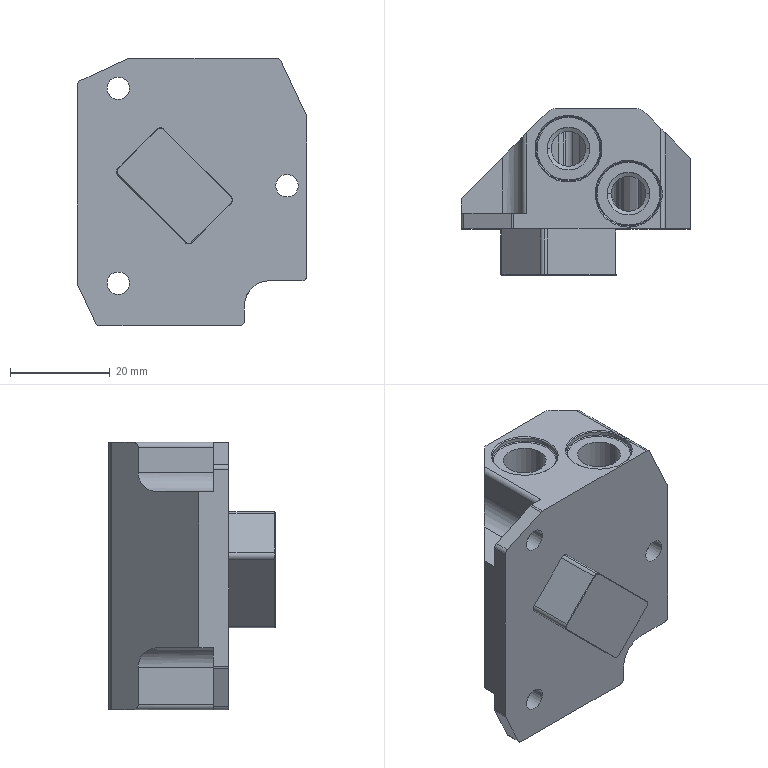NC program | NX | posted with a generic post | part box 46 x 33.25 x 53.5 mm
Lines 4235 to 5331 of 9227:
(CURVE_DRIVE , TOOL : D6R0.5)
N8456 T04 M6
N8458 G53
N8460 G17 G0 G90 X-20.051 Y25.81 B0. C0. S5500 M3
N8462 G43 Z30. H4
N8464 Z-6.42
N8466 G94 G1 Z-7.12 F3000.
N8468 X-20.038 Z-7.382
N8470 X-20.002 Z-7.641
N8472 X-19.944 Z-7.896
N8474 X-19.864 Z-8.145
N8476 X-19.762 Z-8.387
N8478 X-19.64 Z-8.618
N8480 X-19.498 Z-8.838
N8482 X-19.338 Z-9.045
N8484 X-19.16 Z-9.237
N8486 X-18.966 Z-9.412
N8488 X-18.757 Z-9.571
N8490 X-18.536 Z-9.71
N8492 X-18.303 Z-9.829
N8494 X-18.06 Z-9.928
N8496 X-17.81 Z-10.005
N8498 X-17.555 Z-10.061
N8500 X-17.295 Z-10.093
N8502 X-17.033 Z-10.103
N8504 X-3.366
N8506 X-3.309 Y25.792 Z-10.085
N8508 X-3.25 Y25.768 Z-10.061
N8510 X-17.149
N8512 X-17.193 Y25.749 Z-10.042
N8514 X-17.216 Y25.737 Z-10.03
N8516 X-17.234 Y25.726 Z-10.019
N8518 X-3.168 Y25.727 Z-10.02
N8520 X-3.102 Y25.685 Z-9.977
N8522 X-17.302 Y25.684 Z-9.978
N8524 X-17.345 Y25.655 Z-9.948
N8526 X-17.361 Y25.642 Z-9.935
N8528 X-3.043 Y25.643
N8530 X-2.99 Y25.601 Z-9.894
N8532 X-17.412 Y25.6 Z-9.893
N8534 X-17.458 Y25.558 Z-9.851
N8536 X-2.945 Y25.559 Z-9.852
N8538 X-2.918 Y25.532 Z-9.825
N8540 X-2.905 Y25.516 Z-9.81
N8542 X-17.495 Z-9.809
N8544 X-17.531 Y25.474 Z-9.767
N8546 X-2.869
N8548 X-2.855 Y25.456 Z-9.749
N8550 X-2.837 Y25.432 Z-9.725
N8552 X-17.559
N8554 X-17.587 Y25.39 Z-9.683
N8556 X-15.672 Z-9.682
N8558 X-2.809 Z-9.683
N8560 X-2.783 Y25.348 Z-9.641
N8562 X-2.814
N8564 X-17.566 Y25.347
N8566 X-17.615
N8568 X-17.619 Y25.341 Z-9.634
N8570 X-17.638 Y25.305 Z-9.599
N8572 X-17.509 Z-9.598
N8574 X-2.814 Y25.306
N8576 X-2.761 Z-9.599
N8578 X-2.744 Y25.273 Z-9.567
N8580 X-2.74 Y25.263 Z-9.557
N8582 X-2.814 Z-9.556
N8584 X-17.509
N8586 X-17.66
N8588 X-17.676 Y25.221 Z-9.514
N8590 X-17.509
N8592 X-2.814
N8594 X-2.723 Z-9.515
N8596 X-2.715 Y25.202 Z-9.496
N8598 X-2.706 Y25.179 Z-9.474
N8600 X-2.814 Z-9.472
N8602 X-17.509
N8604 X-17.691
N8606 X-17.704 Y25.137 Z-9.43
N8608 X-17.521
N8610 X-2.801
N8612 X-2.695 Z-9.432
N8614 X-2.684 Y25.095 Z-9.389
N8616 X-2.814 Z-9.388
N8618 X-17.558
N8620 X-17.717
N8622 X-17.729 Y25.055 Z-9.348
N8624 X-17.73 Y25.053 Z-9.346
N8626 X-16.499
N8628 X-2.814
N8630 X-2.674 Z-9.347
N8632 X-2.668 Y25.011 Z-9.305
N8634 X-2.814 Z-9.304
N8636 X-17.734
N8638 X-17.739 Y24.968 Z-9.262
N8640 X-2.814 Y24.969
N8642 X-2.662 Z-9.263
N8644 X-2.657 Y24.935 Z-9.229
N8646 Y24.927 Z-9.221
N8648 X-2.814 Z-9.219
N8650 X-17.743 Y24.926
N8652 X-17.745 Y24.884 Z-9.177
N8654 X-2.81
N8656 X-2.655 Z-9.178
N8658 X-2.653 Y24.842 Z-9.136
N8660 X-2.814 Z-9.135
N8662 X-17.747
N8664 X-17.749 Y24.8 Z-9.093
N8666 X-2.814
N8668 X-2.651 Z-9.094
N8670 Y24.758 Z-9.052
N8672 X-2.814 Z-9.051
N8674 X-17.749 Y24.757 Z-9.05
N8676 Y24.715 Z-9.008
N8678 X-2.814
N8680 X-2.651 Z-9.009
N8682 Y24.673 Z-8.967
N8684 X-2.814 Z-8.966
N8686 X-17.749
N8688 Y24.631 Z-8.924
N8690 X-2.814
N8692 X-2.651 Z-8.925
N8694 Y24.588 Z-8.882
N8696 X-2.814 Z-8.881
N8698 X-17.749
N8700 Y24.546 Z-8.839
N8702 X-2.814
N8704 X-2.651 Z-8.84
N8706 Y24.504 Z-8.798
N8708 X-2.814 Z-8.797
N8710 X-17.749 Y24.503 Z-8.796
N8712 Y24.461 Z-8.754
N8714 X-2.814
N8716 X-2.651 Z-8.755
N8718 Y24.419 Z-8.713
N8720 X-2.814 Z-8.712
N8722 X-17.749
N8724 Y24.377 Z-8.67
N8726 X-2.814
N8728 X-2.651 Z-8.671
N8730 Y24.335 Z-8.629
N8732 X-2.814 Z-8.628
N8734 X-17.749 Y24.334 Z-8.627
N8736 Y24.292 Z-8.585
N8738 X-2.814
N8740 X-2.651 Z-8.586
N8742 Y24.25 Z-8.544
N8744 X-2.814 Z-8.543
N8746 X-17.749
N8748 Y24.208 Z-8.501
N8750 X-2.814
N8752 X-2.651 Z-8.502
N8754 Y24.166 Z-8.46
N8756 X-2.814 Z-8.459
N8758 X-17.749 Y24.165 Z-8.458
N8760 Y24.123 Z-8.416
N8762 X-2.814
N8764 X-2.651 Z-8.417
N8766 Y24.081 Z-8.375
N8768 X-2.814 Z-8.374
N8770 X-17.749
N8772 Y24.039 Z-8.332
N8774 X-2.814
N8776 X-2.651 Z-8.333
N8778 Y23.997 Z-8.291
N8780 X-2.814 Z-8.29
N8782 X-17.749 Y23.996 Z-8.289
N8784 Y23.954 Z-8.247
N8786 X-2.814
N8788 X-2.651 Z-8.249
N8790 X-2.65 Y23.912 Z-8.206
N8792 X-2.814 Z-8.205
N8794 X-17.749
N8796 Y23.87 Z-8.163
N8798 X-2.814
N8800 X-2.65 Z-8.164
N8802 Y23.828 Z-8.122
N8804 X-2.814 Z-8.121
N8806 X-17.749 Y23.827 Z-8.12
N8808 Y23.785 Z-8.078
N8810 X-2.814
N8812 X-2.65 Z-8.079
N8814 Y23.743 Z-8.037
N8816 X-2.814 Z-8.036
N8818 X-17.749
N8820 Y23.701 Z-7.994
N8822 X-2.814
N8824 X-2.65 Z-7.995
N8826 Y23.659 Z-7.953
N8828 X-2.814 Z-7.952
N8830 X-17.749 Y23.658 Z-7.951
N8832 Y23.616 Z-7.909
N8834 X-2.814
N8836 X-2.65 Z-7.91
N8838 Y23.574 Z-7.868
N8840 X-2.814 Z-7.867
N8842 X-17.749
N8844 Y23.532 Z-7.825
N8846 X-2.814
N8848 X-2.65 Z-7.826
N8850 Y23.49 Z-7.784
N8852 X-2.814 Y23.489 Z-7.782
N8854 X-17.749
N8856 Y23.447 Z-7.74
N8858 X-2.814
N8860 X-2.65 Z-7.741
N8862 Y23.405 Z-7.699
N8864 X-2.814 Z-7.698
N8866 X-17.749
N8868 Y23.362 Z-7.655
N8870 X-2.814 Y23.363 Z-7.656
N8872 X-2.65 Z-7.657
N8874 Y23.32 Z-7.614
N8876 X-2.814 Z-7.613
N8878 X-17.749
N8880 Y23.278 Z-7.571
N8882 X-2.81 Y23.279
N8884 X-2.65 Z-7.573
N8886 Y23.236 Z-7.53
N8888 X-2.814 Z-7.529
N8890 X-17.749
N8892 Y23.194 Z-7.487
N8894 X-2.814
N8896 X-2.65 Z-7.488
N8898 Y23.152 Z-7.446
N8900 X-2.814 Z-7.445
N8902 X-17.749
N8904 Y23.11 Z-7.403
N8906 X-2.814
N8908 X-2.65 Z-7.404
N8910 Y23.068 Z-7.362
N8912 X-2.814 Z-7.361
N8914 X-17.749
N8916 Y23.026 Z-7.319
N8918 X-2.814
N8920 X-2.65 Z-7.32
N8922 Y22.984 Z-7.278
N8924 X-2.814 Z-7.276
N8926 X-17.749 Y22.983
N8928 Y22.941 Z-7.234
N8930 X-2.814
N8932 X-2.65 Z-7.235
N8934 Y22.899 Z-7.193
N8936 X-2.814 Z-7.192
N8938 X-17.749
N8940 Y22.857 Z-7.15
N8942 X-2.814
N8944 X-2.65 Z-7.151
N8946 Y22.815 Z-7.109
N8948 X-2.814 Z-7.107
N8950 X-17.749 Y22.814
N8952 Y22.772 Z-7.065
N8954 X-2.814
N8956 X-2.65 Z-7.066
N8958 Y22.73 Z-7.024
N8960 X-2.814 Z-7.023
N8962 X-17.749
N8964 Y22.687 Z-6.98
N8966 X-2.814 Y22.688
N8968 X-2.65 Z-6.982
N8970 Y22.645 Z-6.939
N8972 X-2.814 Z-6.938
N8974 X-17.749
N8976 X-17.75 Y22.603 Z-6.896
N8978 X-2.814
N8980 X-2.65 Z-6.897
N8982 Y22.561 Z-6.855
N8984 X-2.814 Y22.56 Z-6.853
N8986 X-17.75
N8988 Y22.518 Z-6.811
N8990 X-2.814
N8992 X-2.65 Z-6.812
N8994 Y22.476 Z-6.77
N8996 X-2.814 Z-6.769
N8998 X-17.75
N9000 Y22.433 Z-6.726
N9002 X-2.814 Y22.434 Z-6.727
N9004 X-2.65 Z-6.728
N9006 Y22.391 Z-6.685
N9008 X-2.814 Z-6.684
N9010 X-17.75
N9012 Y22.349 Z-6.642
N9014 X-2.814
N9016 X-2.649 Z-6.643
N9018 Y22.307 Z-6.601
N9020 X-2.814 Z-6.6
N9022 X-17.75
N9024 Y22.264 Z-6.557
N9026 X-2.814 Y22.265
N9028 X-2.649 Z-6.559
N9030 Y22.222 Z-6.516
N9032 X-2.814 Z-6.515
N9034 X-17.75
N9036 Y22.18 Z-6.473
N9038 X-2.814
N9040 X-2.649 Z-6.474
N9042 Y22.138 Z-6.432
N9044 X-2.814 Z-6.431
N9046 X-17.75
N9048 Y22.095 Z-6.388
N9050 X-2.814
N9052 X-2.649 Z-6.39
N9054 Y22.053 Z-6.347
N9056 X-2.814 Z-6.346
N9058 X-17.75
N9060 Y22.011 Z-6.304
N9062 X-2.814
N9064 X-2.649 Z-6.305
N9066 Y21.969 Z-6.263
N9068 X-2.814 Z-6.262
N9070 X-17.75 Y21.968 Z-6.261
N9072 Y21.926 Z-6.219
N9074 X-2.814
N9076 X-2.648 Z-6.22
N9078 X-2.647 Y21.884 Z-6.178
N9080 X-2.814 Z-6.177
N9082 X-17.75
N9084 Y21.842 Z-6.135
N9086 X-2.814
N9088 X-2.646 Z-6.136
N9090 X-2.645 Y21.8 Z-6.094
N9092 X-2.814 Z-6.092
N9094 X-17.75 Y21.799
N9096 Y21.757 Z-6.05
N9098 X-2.814
N9100 X-2.645 Z-6.051
N9102 X-2.644 Y21.728 Z-6.022
N9104 X-2.643 Y21.715 Z-6.009
N9106 X-2.814 Z-6.008
N9108 X-17.75
N9110 Y21.672 Z-5.965
N9112 X-2.807 Y21.673 Z-5.966
N9114 X-2.64 Z-5.967
N9116 X-2.638 Y21.63 Z-5.924
N9118 X-2.814 Z-5.923
N9120 X-17.75
N9122 Y21.588 Z-5.881
N9124 X-2.721
N9126 X-2.635 Z-5.882
N9128 X-2.632 Y21.546 Z-5.839
N9130 X-2.814
N9132 X-17.75 Y21.545 Z-5.838
N9134 Y21.503 Z-5.796
N9136 X-2.814
N9138 X-2.629 Z-5.797
N9140 X-2.626 Y21.461 Z-5.755
N9142 X-2.814 Z-5.754
N9144 X-17.75
N9146 Y21.419 Z-5.712
N9148 X-2.814
N9150 X-2.621 Z-5.713
N9152 X-2.615 Y21.377 Z-5.671
N9154 X-2.814 Z-5.67
N9156 X-17.75
N9158 Y21.334 Z-5.627
N9160 X-2.814 Y21.335 Z-5.628
N9162 X-2.609
N9164 X-2.604 Y21.293 Z-5.586
N9166 X-2.814
N9168 X-17.75 Y21.292 Z-5.585
N9170 Y21.25 Z-5.543
N9172 X-2.814 Y21.251 Z-5.544
N9174 X-2.598
N9176 X-2.592 Y21.209 Z-5.502
N9178 X-6.488 Y21.208 Z-5.501
N9180 X-17.75
N9182 Y21.166 Z-5.459
N9184 X-2.585 Z-5.46
N9186 X-2.576 Y21.124 Z-5.417
N9188 X-17.75
N9190 Y21.082 Z-5.375
N9192 X-2.567
N9194 X-2.558 Y21.04 Z-5.333
N9196 X-17.75 Y21.039 Z-5.332
N9198 Y20.997 Z-5.29
N9200 X-2.549 Y20.998 Z-5.291
N9202 X-2.541 Y20.955 Z-5.248
N9204 X-17.75
N9206 Y20.913 Z-5.206
N9208 X-2.531
N9210 X-2.519 Y20.871 Z-5.164
N9212 X-3.477
N9214 X-17.75
N9216 Y20.829 Z-5.122
N9218 X-2.508
N9220 X-2.496 Y20.787 Z-5.08
N9222 X-17.75 Y20.786 Z-5.079
N9224 Y20.744 Z-5.037
N9226 X-2.484
N9228 X-2.473 Y20.702 Z-4.995
N9230 X-17.75
N9232 Y20.66 Z-4.953
N9234 X-2.461
N9236 X-2.447 Y20.618 Z-4.911
N9238 X-17.75 Y20.617 Z-4.91
N9240 Y20.575 Z-4.868
N9242 X-2.432
N9244 X-2.417 Y20.533 Z-4.826
N9246 X-17.75
N9248 Y20.49 Z-4.783
N9250 X-2.403 Y20.491 Z-4.784
N9252 X-2.386 Y20.448 Z-4.742
N9254 X-4.417 Z-4.741
N9256 X-17.75
N9258 Y20.406 Z-4.699
N9260 X-2.488
N9262 X-2.369
N9264 X-2.363 Y20.392 Z-4.685
N9266 X-2.351 Y20.363 Z-4.657
N9268 X-2.538 Z-4.656
N9270 X-17.75
N9272 Y20.321 Z-4.614
N9274 X-2.521
N9276 X-2.332 Z-4.615
N9278 X-2.312 Y20.279 Z-4.572
N9280 X-2.479
N9282 X-17.75
N9284 Y20.236 Z-4.529
N9286 X-2.437 Y20.237 Z-4.53
N9288 X-2.293
N9290 X-2.274 Y20.194 Z-4.488
N9292 X-12.786 Z-4.487
N9294 X-17.75
N9296 Y20.152 Z-4.445
N9298 X-2.28
N9300 X-2.255
N9302 X-2.243 Y20.125 Z-4.418
N9304 X-2.235 Y20.11 Z-4.403
N9306 X-2.31
N9308 X-17.75 Y20.109 Z-4.402
N9310 Y20.067 Z-4.36
N9312 X-2.268
N9314 X-2.214 Z-4.361
N9316 X-2.193 Y20.025 Z-4.318
N9318 X-17.75
N9320 Y19.983 Z-4.276
N9322 X-2.172
N9324 X-2.148 Y19.941 Z-4.234
N9326 X-17.75 Y19.94 Z-4.233
N9328 Y19.898 Z-4.191
N9330 X-2.124 Z-4.192
N9332 X-2.098 Y19.856 Z-4.149
N9334 X-3.231
N9336 X-17.75
N9338 Y19.813 Z-4.106
N9340 X-2.277 Y19.814 Z-4.107
N9342 X-2.072
N9344 X-2.045 Y19.771 Z-4.065
N9346 X-2.238 Z-4.064
N9348 X-17.75
N9350 Y19.729 Z-4.022
N9352 X-2.196
N9354 X-2.018 Z-4.023
N9356 X-1.99 Y19.687 Z-3.981
N9358 X-2.154 Z-3.98
N9360 X-17.75
N9362 Y19.645 Z-3.938
N9364 X-2.012
N9366 X-1.962 Z-3.939
N9368 X-1.933 Y19.603 Z-3.897
N9370 X-2.012 Z-3.896
N9372 X-17.75 Y19.602 Z-3.895
N9374 Y19.56 Z-3.853
N9376 X-2.012
N9378 X-1.904 Z-3.855
N9380 X-1.872 Y19.518 Z-3.813
N9382 X-1.985 Z-3.811
N9384 X-17.75
N9386 Y19.476 Z-3.769
N9388 X-1.873 Z-3.77
N9390 X-1.839
N9392 X-1.807 Y19.434 Z-3.727
N9394 X-17.75
N9396 Y19.392 Z-3.685
N9398 X-1.772
N9400 X-1.737 Y19.35 Z-3.643
N9402 X-17.75 Y19.349 Z-3.642
N9404 Y19.307 Z-3.6
N9406 X-1.702 Z-3.601
N9408 X-1.666 Y19.265 Z-3.558
N9410 X-17.75
N9412 Y19.222 Z-3.515
N9414 X-1.628 Y19.223 Z-3.516
N9416 X-1.588 Y19.18 Z-3.474
N9418 X-17.75 Z-3.473
N9420 Y19.138 Z-3.431
N9422 X-1.548
N9424 X-1.505 Y19.096 Z-3.389
N9426 X-11.529
N9428 X-17.75
N9430 Y19.053 Z-3.346
N9432 X-1.499 Y19.054 Z-3.347
N9434 X-1.463
N9436 X-1.418 Y19.011 Z-3.305
N9438 X-1.476 Z-3.304
N9440 X-17.75
N9442 Y18.969 Z-3.262
N9444 X-1.373
N9446 X-1.35 Y18.949 Z-3.242
N9448 X-1.325 Y18.927 Z-3.22
N9450 X-17.75
N9452 Y18.884 Z-3.177
N9454 X-1.277 Y18.885 Z-3.178
N9456 X-1.264 Y18.874 Z-3.167
N9458 X-1.226 Y18.842 Z-3.136
N9460 X-17.75 Z-3.135
N9462 Y18.8 Z-3.093
N9464 X-1.175
N9466 X-1.16 Y18.788 Z-3.081
N9468 X-1.12 Y18.758 Z-3.051
N9470 X-17.75 Y18.757 Z-3.05
N9472 X-17.751 Y18.715 Z-3.008
N9474 X-1.063
N9476 X-1.004 Y18.673 Z-2.966
N9478 X-17.751
N9480 Y18.631 Z-2.924
N9482 X-0.963
N9484 X-0.944 Z-2.925
N9486 X-0.881 Y18.589 Z-2.882
N9488 X-17.751
N9490 Y18.547 Z-2.84
N9492 X-0.817
N9494 X-0.774 Y18.521 Z-2.814
N9496 X-0.745 Y18.505 Z-2.798
N9498 X-17.751
N9500 Y18.462 Z-2.755
N9502 X-0.67 Y18.463 Z-2.756
N9504 X-0.595 Y18.421 Z-2.714
N9506 X-17.752 Y18.42 Z-2.713
N9508 X-17.753 Y18.379 Z-2.671
N9510 X-0.515 Z-2.672
N9512 X-0.434 Y18.338 Z-2.631
N9514 X-17.753 Y18.337 Z-2.63
N9516 X-17.754 Y18.296 Z-2.589
N9518 X-0.343
N9520 X-0.29 Y18.272 Z-2.565
N9522 X-0.25 Y18.254 Z-2.547
N9524 X-17.755
N9526 X-17.756 Y18.214 Z-2.507
N9528 X-0.147
N9530 X-0.033 Y18.172 Z-2.465
N9532 X-17.758
N9534 X-17.76 Y18.13 Z-2.423
N9536 X0.022
N9538 X0.096
N9540 X0.109 Y18.125 Z-2.419
N9542 X0.244 Y18.088 Z-2.381
N9544 X-17.762
N9546 X-17.764 Y18.048 Z-2.341
N9548 X0.289
N9550 X0.415 Z-2.342
N9552 X0.512 Y18.026 Z-2.32
N9554 X0.6 Y18.009 Z-2.303
N9556 X0.526 Z-2.302
N9558 X0.392 Z-2.303
N9560 X0.328 Z-2.302
N9562 X-17.766
N9564 X-17.767 Y17.987 Z-2.28
N9566 X-17.769 Y17.967 Z-2.26
N9568 X0.615
N9570 X0.659 Z-2.261
N9572 X0.793 Z-2.26
N9574 X0.945 Z-2.261
N9576 X1.207 Z-2.249
N9578 X1.466 Z-2.215
N9580 X1.722 Z-2.159
N9582 X1.971 Z-2.08
N9584 X2.213 Z-1.98
N9586 X2.445 Z-1.859
N9588 X2.666 Z-1.718
N9590 X2.874 Z-1.559
N9592 X3.067 Z-1.382
N9594 X3.244 Z-1.189
N9596 X3.403 Z-0.982
N9598 X3.544 Z-0.761
N9600 X3.664 Z-0.529
N9602 X3.765 Z-0.287
N9604 X3.843 Z-0.037
N9606 X3.9 Z0.218
N9608 X3.934 Z0.478
N9610 X3.945 Z0.739
N9612 Z1.899
N9614 G0 Z4.489
N9616 X2.869 Y25.81
N9618 Z-6.411
N9620 G1 Z-7.103
N9622 X2.88 Z-7.365
N9624 X2.914 Z-7.624
N9626 X2.971 Z-7.88
N9628 X3.05 Z-8.129
N9630 X3.15 Z-8.371
N9632 X3.271 Z-8.603
N9634 X3.411 Z-8.824
N9636 X3.571 Z-9.032
N9638 X3.747 Z-9.225
N9640 X3.94 Y25.811 Z-9.402
N9642 X4.148 Z-9.561
N9644 X4.369 Z-9.701
N9646 X4.601 Z-9.822
N9648 X4.843 Z-9.923
N9650 X5.092 Z-10.001
N9652 X5.348 Z-10.058
N9654 X5.607 Z-10.092
N9656 X5.869 Z-10.103
N9658 X15.11 Z-10.104
N9660 X15.135 Y25.803 Z-10.096
N9662 X15.201 Y25.779 Z-10.073
N9664 X15.227 Y25.769 Z-10.062
N9666 X5.822 Y25.768 Z-10.061
N9668 X5.757 Z-10.063
N9670 X5.685 Y25.737 Z-10.031
N9672 X5.668 Y25.727 Z-10.021
N9674 X5.78 Z-10.02
N9676 X15.268
N9678 X15.321
N9680 X15.411 Y25.685 Z-9.978
N9682 X5.738
N9684 X5.598 Z-9.979
N9686 X5.54 Y25.643 Z-9.937
N9688 X5.653 Z-9.936
N9690 X15.501
N9692 X15.591 Y25.601 Z-9.894
N9694 X5.569
N9696 X5.49
N9698 X5.478 Y25.591 Z-9.885
N9700 X5.445 Y25.559 Z-9.852
N9702 X5.485
N9704 X15.681
N9706 X15.771 Y25.517 Z-9.81
N9708 X5.469
N9710 X5.405
N9712 X5.368 Y25.474 Z-9.768
N9714 X5.469 Z-9.767
N9716 X15.862 Y25.475 Z-9.768
N9718 X15.953 Y25.432 Z-9.725
N9720 X5.469
N9722 X5.337 Z-9.726
N9724 X5.311 Y25.39 Z-9.684
N9726 X5.442 Z-9.683
N9728 X16.043
N9730 X16.133 Y25.348 Z-9.641
N9732 X5.33
N9734 X5.286
N9736 X5.272 Y25.324 Z-9.617
N9738 X5.263 Y25.306 Z-9.599
N9740 X16.224
N9742 X16.314 Y25.264 Z-9.557
N9744 X5.244 Y25.263
N9746 X5.225 Y25.221 Z-9.514
N9748 X16.352
N9750 X16.404 Z-9.516
N9752 X16.494 Y25.179 Z-9.474
N9754 X16.394 Z-9.472
N9756 X5.21
N9758 X5.197 Y25.137 Z-9.43
N9760 X16.585 Z-9.431
N9762 X16.674 Y25.095 Z-9.389
N9764 X16.612 Z-9.388
N9766 X5.185
N9768 X5.178 Y25.071 Z-9.364
N9770 X5.175 Y25.053 Z-9.346
N9772 X16.654
N9774 X16.764 Z-9.347
N9776 X16.855 Y25.011 Z-9.305
N9778 X16.701 Z-9.304
N9780 X5.169
N9782 X5.162 Y24.969 Z-9.262
N9784 X16.786
N9786 X16.945 Z-9.263
N9788 X17.036 Y24.927 Z-9.221
N9790 X16.87 Z-9.22
N9792 X5.202
N9794 X5.157
N9796 X5.155 Y24.885 Z-9.178
N9798 X5.203 Z-9.177
N9800 X17.127 Z-9.178
N9802 X17.217 Y24.843 Z-9.136
N9804 X17.132 Z-9.135
N9806 X5.202 Y24.842
N9808 X5.153 Z-9.136
N9810 X5.151 Y24.8 Z-9.093
N9812 X5.202
N9814 X17.174
N9816 X17.307 Z-9.094
N9818 X17.398 Y24.758 Z-9.052
N9820 X17.219 Z-9.051
N9822 X5.202
N9824 X5.151
N9826 Y24.716 Z-9.009
N9828 X5.202 Z-9.008
N9830 X17.293 Z-9.009
N9832 X17.489
N9834 X17.58 Y24.673 Z-8.967
N9836 X17.378 Z-8.966
N9838 X5.202
N9840 X5.151 Z-8.967
N9842 Y24.631 Z-8.924
N9844 X5.202
N9846 X17.67
N9848 X17.761 Y24.589 Z-8.882
N9850 X12.9
N9852 X5.202 Z-8.881
N9854 X5.151 Z-8.882
N9856 Y24.546 Z-8.84
N9858 X5.202 Z-8.839
N9860 X17.852 Z-8.84
N9862 X17.943 Y24.504 Z-8.797
N9864 X5.202
N9866 X5.151
N9868 Y24.462 Z-8.755
N9870 X5.202 Z-8.754
N9872 X18.034 Z-8.755
N9874 X18.125 Y24.42 Z-8.713
N9876 X5.202 Y24.419 Z-8.712
N9878 X5.151 Z-8.713
N9880 Y24.377 Z-8.67
N9882 X5.202
N9884 X18.215
N9886 X18.306 Y24.335 Z-8.628
N9888 X5.202
N9890 X5.151
N9892 Y24.293 Z-8.586
N9894 X5.202 Z-8.585
N9896 X18.397 Z-8.586
N9898 X18.487 Y24.251 Z-8.543
N9900 X5.202 Y24.25
N9902 X5.151 Z-8.544
N9904 Y24.208 Z-8.501
N9906 X5.202
N9908 X18.578
N9910 X18.668 Y24.166 Z-8.459
N9912 X5.202
N9914 X5.151
N9916 Y24.124 Z-8.417
N9918 X5.202 Z-8.416
N9920 X18.759 Z-8.417
N9922 X18.849 Y24.082 Z-8.375
N9924 X5.203 Y24.081 Z-8.374
N9926 X5.151 Z-8.375
N9928 Y24.039 Z-8.332
N9930 X5.202
N9932 X18.94 Z-8.333
N9934 X19.03 Y23.997 Z-8.29
N9936 X5.202
N9938 X5.151
N9940 Y23.955 Z-8.248
N9942 X5.202
N9944 X19.121
N9946 X19.211 Y23.913 Z-8.206
N9948 X5.202 Y23.912 Z-8.205
N9950 X5.15 Z-8.206
N9952 Y23.87 Z-8.163
N9954 X5.202
N9956 X19.253
N9958 X19.302 Z-8.164
N9960 X19.393 Y23.828 Z-8.121
N9962 X6.969
N9964 X5.202
N9966 X5.15
N9968 Y23.786 Z-8.079
N9970 X5.202 Z-8.078
N9972 X19.483 Z-8.079
N9974 X19.574 Y23.744 Z-8.037
N9976 X5.202 Y23.743 Z-8.036
N9978 X5.15 Z-8.037
N9980 Y23.701 Z-7.994
N9982 X5.202
N9984 X19.665
N9986 X19.755 Y23.659 Z-7.952
N9988 X5.202
N9990 X5.15
N9992 Y23.616 Z-7.91
N9994 X5.202 Z-7.909
N9996 X19.846 Y23.617 Z-7.91
N9998 X19.937 Y23.574 Z-7.868
N10000 X5.202 Z-7.867
N10002 X5.15 Z-7.868
N10004 Y23.532 Z-7.825
N10006 X5.202
N10008 X20.028
N10010 X20.118 Y23.49 Z-7.783
N10012 X5.202
N10014 X5.15
N10016 Y23.447 Z-7.741
N10018 X5.202 Z-7.74
N10020 X20.209 Y23.448 Z-7.741
N10022 X20.3 Y23.405 Z-7.698
N10024 X5.202
N10026 X5.15
N10028 Y23.363 Z-7.656
N10030 X5.202
N10032 X20.35
N10034 X20.389 Z-7.657
N10036 X20.479 Y23.321 Z-7.615
N10038 X20.392 Z-7.614
N10040 X5.202 Z-7.613
N10042 X5.15 Z-7.614
N10044 Y23.279 Z-7.572
N10046 X5.205
N10048 X20.571
N10050 X20.66 Y23.237 Z-7.531
N10052 X20.61 Z-7.53
N10054 X5.202 Y23.236 Z-7.529
N10056 X5.15 Z-7.53
N10058 Y23.194 Z-7.488
N10060 X5.202 Z-7.487
N10062 X20.652 Y23.195 Z-7.488
N10064 X20.75 Z-7.489
N10066 X20.841 Y23.153 Z-7.447
N10068 X20.694 Z-7.446
N10070 X5.202 Y23.152 Z-7.445
N10072 X5.15 Z-7.446
N10074 Y23.11 Z-7.404
N10076 X5.202 Z-7.403
N10078 X20.774 Y23.111
N10080 X20.931 Z-7.405
N10082 X21.021 Y23.068 Z-7.362
N10084 X20.859 Z-7.361
N10086 X5.202
N10088 X5.15
N10090 Y23.026 Z-7.319
N10092 X5.202
N10094 X21.099
N10096 X21.112 Z-7.32
N10098 X21.203 Y22.984 Z-7.278
N10100 X21.13 Z-7.277
N10102 X5.202
N10104 X5.15
N10106 Y22.941 Z-7.235
N10108 X5.202 Z-7.234
N10110 X21.172 Y22.942 Z-7.235
N10112 X21.293
N10114 X21.384 Y22.9 Z-7.193
N10116 X21.215 Z-7.192
N10118 X5.202 Y22.899
N10120 X5.15 Z-7.193
N10122 Y22.857 Z-7.15
N10124 X5.202
N10126 X21.282
N10128 X21.474 Z-7.151
N10130 X21.565 Y22.815 Z-7.108
N10132 X21.366
N10134 X5.202
N10136 X5.15
N10138 Y22.772 Z-7.066
N10140 X5.202 Z-7.065
N10142 X21.5 Y22.773 Z-7.066
N10144 X21.656
N10146 X21.747 Y22.73 Z-7.024
N10148 X18.458 Z-7.023
N10150 X5.202
N10152 X5.15
N10154 Y22.688 Z-6.981
N10156 X5.202
N10158 X21.838
N10160 X21.929 Y22.646 Z-6.939
N10162 X5.202 Y22.645 Z-6.938
N10164 X5.15 Z-6.939
N10166 Y22.603 Z-6.896
N10168 X5.202
N10170 X22.02
N10172 X22.11 Y22.561 Z-6.854
N10174 X5.202
N10176 X5.15
N10178 Y22.518 Z-6.812
N10180 X5.202 Z-6.811
N10182 X22.201 Y22.519 Z-6.812
N10184 X22.292 Y22.476 Z-6.769
N10186 X5.202
N10188 X5.15
N10190 Y22.434 Z-6.727
N10192 X5.202
N10194 X22.383
N10196 X22.473 Y22.392 Z-6.685
N10198 X5.202 Z-6.684
N10200 X5.149 Z-6.685
N10202 Y22.349 Z-6.643
N10204 X5.202 Z-6.642
N10206 X22.564 Y22.35
N10208 X22.654 Y22.307 Z-6.6
N10210 X5.202
N10212 X5.149
N10214 Y22.265 Z-6.558
N10216 X5.202
N10218 X22.745
N10220 X22.836 Y22.223 Z-6.516
N10222 X5.202 Y22.222 Z-6.515
N10224 X5.149 Z-6.516
N10226 Y22.18 Z-6.474
N10228 X5.202 Z-6.473
N10230 X22.926 Z-6.474
N10232 X23.017 Y22.138 Z-6.431
N10234 X5.202
N10236 X5.149
N10238 Y22.096 Z-6.389
N10240 X5.202
N10242 X23.075
N10244 X23.107
N10246 X23.198 Y22.054 Z-6.347
N10248 X5.202 Y22.053 Z-6.346
N10250 X5.149 Z-6.347
N10252 Y22.011 Z-6.304
N10254 X5.202
N10256 X23.289 Z-6.305
N10258 X23.379 Y21.969 Z-6.262
N10260 X23.327
N10262 X5.202
N10264 X5.149
N10266 X5.148 Y21.927 Z-6.22
N10268 X5.202 Z-6.219
N10270 X23.47 Z-6.22
N10272 X23.561 Y21.885 Z-6.178
N10274 X5.202 Y21.884 Z-6.177
N10276 X5.147 Z-6.178
N10278 X5.146 Y21.842 Z-6.135
N10280 X5.202
N10282 X23.651 Z-6.136
N10284 X23.742 Y21.8 Z-6.093
N10286 X5.202
N10288 X5.145
N10290 X5.144 Y21.757 Z-6.051
N10292 X5.202 Z-6.05
N10294 X23.833 Y21.758 Z-6.051
N10296 X23.924 Y21.715 Z-6.008
N10298 X5.202
N10300 X5.143
N10302 X5.14 Y21.673 Z-5.966
N10304 X5.202
N10306 X24.015
N10308 X24.105 Y21.631 Z-5.924
N10310 X5.184 Y21.63 Z-5.923
N10312 X5.138 Z-5.924
N10314 X5.135 Y21.588 Z-5.881
N10316 X24.196
N10318 X24.287 Y21.546 Z-5.839
N10320 X5.132
N10322 X5.13 Y21.504 Z-5.797
N10324 X24.349
N10326 X24.377 Z-5.798
N10328 X24.467 Y21.462 Z-5.756
N10330 X24.391 Z-5.754
N10332 X5.127 Y21.461
N10334 X5.122 Y21.419 Z-5.713
N10336 X24.558 Y21.42
N10338 X24.648 Y21.377 Z-5.671
N10340 X24.609 Z-5.67
N10342 X5.116
N10344 X5.11 Y21.335 Z-5.628
N10346 X11.28
N10348 X24.651
N10350 X24.738 Z-5.629
N10352 X24.828 Y21.293 Z-5.587
N10354 X24.693 Z-5.586
N10356 X5.129
N10358 X5.105
N10360 X5.099 Y21.251 Z-5.545
N10362 X5.202 Z-5.544
N10364 X24.765
N10366 X24.918 Z-5.545
N10368 X25.009 Y21.209 Z-5.503
N10370 X24.849 Z-5.502
N10372 X5.171
N10374 X5.093 Z-5.503
N10376 X5.087 Y21.167 Z-5.461
N10378 X5.202 Z-5.459
N10380 X24.973 Z-5.46
N10382 X25.1
N10384 X25.19 Y21.125 Z-5.418
N10386 X25.129
N10388 X5.202 Y21.124 Z-5.417
N10390 X5.08 Z-5.419
N10392 X5.073 Y21.082 Z-5.377
N10394 X5.202 Z-5.375
N10396 X25.171
N10398 X25.28 Z-5.376
N10400 X25.371 Y21.04 Z-5.334
N10402 X25.214 Z-5.333
N10404 X5.202
N10406 X5.063 Z-5.335
N10408 X5.052 Y20.998 Z-5.292
N10410 X5.202 Z-5.291
N10412 X25.272
N10414 X25.462 Z-5.292
N10416 X25.552 Y20.956 Z-5.249
N10418 X25.356
N10420 X5.202 Y20.955 Z-5.248
N10422 X5.042 Z-5.25
N10424 X5.031 Y20.913 Z-5.207
N10426 X5.202 Z-5.206
N10428 X25.507 Y20.914 Z-5.207
N10430 X25.643
N10432 X25.733 Y20.872 Z-5.165
N10434 X22.976 Y20.871 Z-5.164
N10436 X5.193
N10438 X5.019 Z-5.165
N10440 X5.007 Y20.829 Z-5.123
N10442 X5.152 Z-5.122
N10444 X25.558
N10446 X25.824 Z-5.123
N10448 X25.914 Y20.787 Z-5.08
N10450 X5.111
N10452 X4.995
N10454 X4.983 Y20.745 Z-5.038
N10456 X5.07
N10458 X26.005
N10460 X26.094 Y20.703 Z-4.996
N10462 X4.971 Y20.702
N10464 X4.959 Y20.66 Z-4.953
N10466 X26.183 Z-4.954
N10468 X26.261 Y20.618 Z-4.911
N10470 X4.944
N10472 X4.929 Y20.575 Z-4.868
N10474 X26.325 Y20.576 Z-4.869
N10476 X26.337 Y20.568 Z-4.861
N10478 X26.38 Y20.533 Z-4.827
N10480 X4.913 Z-4.826
N10482 X4.898 Y20.491 Z-4.784
N10484 X26.429
N10486 X26.466 Y20.455 Z-4.748
N10488 X26.473 Y20.449 Z-4.742
N10490 X4.883 Y20.448 Z-4.741
N10492 X4.868 Y20.406 Z-4.699
N10494 X26.512
N10496 X26.525 Y20.392 Z-4.685
N10498 X26.534 Y20.381 Z-4.674
N10500 X26.545 Y20.364 Z-4.657
N10502 X4.851
N10504 X4.833 Y20.321 Z-4.615
N10506 X26.572 Y20.322
N10508 X26.599 Y20.28 Z-4.573
N10510 X4.816 Y20.279 Z-4.572
N10512 X4.804 Y20.252 Z-4.545
N10514 X4.797 Y20.237 Z-4.53
N10516 X26.576
N10518 X26.623 Z-4.531
N10520 X26.644 Y20.195 Z-4.489
N10522 X26.576 Z-4.488
N10524 X4.777 Y20.194
N10526 X4.757 Y20.152 Z-4.445
N10528 X26.576 Y20.153
N10530 X26.664 Z-4.447
N10532 X26.678 Y20.124 Z-4.418
N10534 X26.682 Y20.11 Z-4.405
N10536 X26.576 Z-4.403
N10538 X4.934
N10540 X4.736
N10542 X4.714 Y20.067 Z-4.361
N10544 X6.287 Z-4.36
N10546 X26.588 Y20.068 Z-4.361
N10548 X26.696 Z-4.362
N10550 X26.709 Y20.026 Z-4.32
N10552 X26.576 Z-4.318
N10554 X4.692 Y20.025
N10556 X4.67 Y19.983 Z-4.276
N10558 X26.576
N10560 X26.721 Z-4.277
N10562 X26.728 Y19.941 Z-4.235
N10564 X26.576 Z-4.234
N10566 X4.646
N10568 X4.622 Y19.898 Z-4.192
N10570 X26.576 Y19.899
N10572 X26.735 Z-4.193
N10574 X26.742 Y19.856 Z-4.15
N10576 X26.576 Z-4.149
N10578 X4.598
N10580 X4.572 Y19.814 Z-4.107
N10582 X26.581
N10584 X26.744 Z-4.108
N10586 X26.746 Y19.772 Z-4.066
N10588 X26.576 Z-4.065
N10590 X4.546
N10592 X4.536 Y19.756 Z-4.049
N10594 X4.518 Y19.729 Z-4.023
N10596 X26.576 Y19.73
N10598 X26.748 Z-4.024
N10600 X26.749 Y19.688 Z-3.982
N10602 X26.576 Z-3.981
N10604 X4.489 Y19.687 Z-3.98
N10606 X4.46 Y19.645 Z-3.938
N10608 X26.576 Y19.646
N10610 X26.749 Z-3.939
N10612 Y19.603 Z-3.897
N10614 X26.576 Z-3.896
N10616 X4.43
N10618 X4.422 Y19.59 Z-3.883
N10620 X4.4 Y19.561 Z-3.854
N10622 X26.576
N10624 X26.749 Z-3.855
N10626 Y19.519 Z-3.813
N10628 X26.576 Z-3.812
N10630 X4.368 Y19.518 Z-3.811
N10632 X4.337 Y19.477 Z-3.77
N10634 X26.576
N10636 X26.749 Z-3.771
N10638 Y19.435 Z-3.729
N10640 X26.576 Z-3.728
N10642 X4.305 Y19.434 Z-3.727